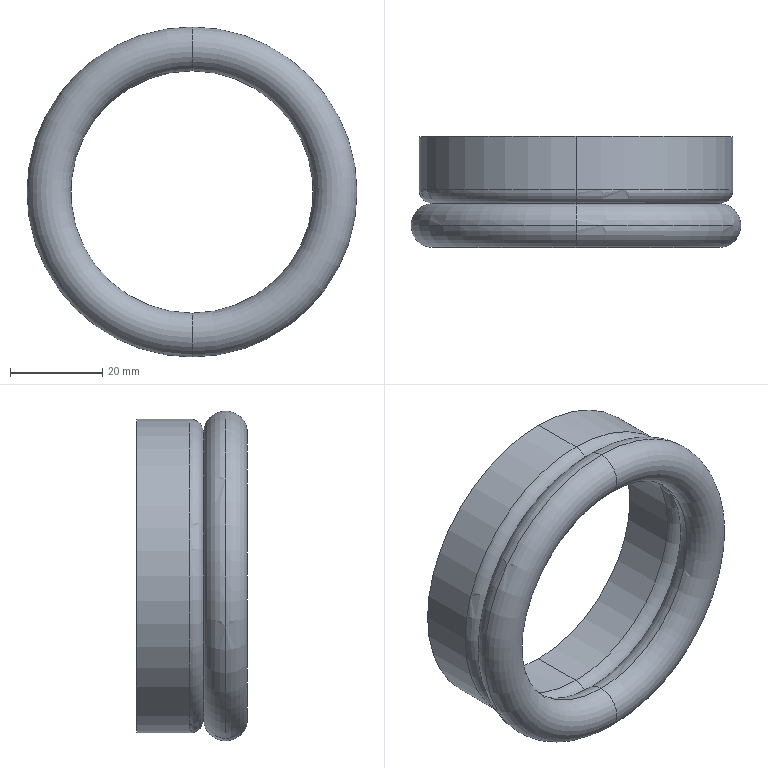Part | SolidWorks | features Sweep 2 | 2 solids | 22 faces | box 71.5 x 24 x 71.5 mm | volume 15845 mm3 | torus 12 | cylinder 8 | plane 2 | commonest cylinder face diameters 56 x2 59.2 x2 64.8 x2 68 x2
STEP:
#1=CARTESIAN_POINT('',(31.,19.25,32.4));
#2=VERTEX_POINT('',#1);
#3=CARTESIAN_POINT('',(31.,19.25,-32.4));
#4=VERTEX_POINT('',#3);
#5=CARTESIAN_POINT('',(31.,19.25,0.));
#6=DIRECTION('',(0.,-1.,0.));
#7=DIRECTION('',(0.,0.,-1.));
#8=AXIS2_PLACEMENT_3D('',#5,#6,#7);
#9=CIRCLE('',#8,32.4);
#10=EDGE_CURVE('',#2,#4,#9,.T.);
#11=ORIENTED_EDGE('',*,*,#10,.F.);
#12=CARTESIAN_POINT('',(31.,7.75,32.4));
#13=VERTEX_POINT('',#12);
#14=CARTESIAN_POINT('',(31.,0.,32.4));
#15=DIRECTION('',(0.,-1.,0.));
#16=VECTOR('',#15,1000.);
#17=LINE('',#14,#16);
#18=EDGE_CURVE('',#2,#13,#17,.T.);
#19=ORIENTED_EDGE('',*,*,#18,.T.);
#20=CARTESIAN_POINT('',(31.,7.75,-32.4));
#21=VERTEX_POINT('',#20);
#22=CARTESIAN_POINT('',(31.,7.75,0.));
#23=DIRECTION('',(0.,-1.,0.));
#24=DIRECTION('',(0.,0.,-1.));
#25=AXIS2_PLACEMENT_3D('',#22,#23,#24);
#26=CIRCLE('',#25,32.4);
#27=EDGE_CURVE('',#13,#21,#26,.T.);
#28=ORIENTED_EDGE('',*,*,#27,.T.);
#29=CARTESIAN_POINT('',(31.,0.,-32.4));
#30=DIRECTION('',(0.,-1.,0.));
#31=VECTOR('',#30,1000.);
#32=LINE('',#29,#31);
#33=EDGE_CURVE('',#4,#21,#32,.T.);
#34=ORIENTED_EDGE('',*,*,#33,.F.);
#35=EDGE_LOOP('',(#11,#19,#28,#34));
#36=FACE_OUTER_BOUND('',#35,.T.);
#37=CARTESIAN_POINT('',(31.,0.,0.));
#38=DIRECTION('',(0.,-1.,0.));
#39=DIRECTION('',(0.,0.,-1.));
#40=AXIS2_PLACEMENT_3D('',#37,#38,#39);
#41=CYLINDRICAL_SURFACE('',#40,32.4);
#42=ADVANCED_FACE('',(#36),#41,.F.);
#43=ORIENTED_EDGE('',*,*,#27,.F.);
#44=CARTESIAN_POINT('',(31.,7.75,29.6));
#45=VERTEX_POINT('',#44);
#46=CARTESIAN_POINT('',(31.,7.75,31.));
#47=DIRECTION('',(1.,0.,0.));
#48=DIRECTION('',(0.,0.,-1.));
#49=AXIS2_PLACEMENT_3D('',#46,#47,#48);
#50=CIRCLE('',#49,1.4);
#51=EDGE_CURVE('',#13,#45,#50,.T.);
#52=ORIENTED_EDGE('',*,*,#51,.T.);
#53=CARTESIAN_POINT('',(31.,7.75,-29.6));
#54=VERTEX_POINT('',#53);
#55=CARTESIAN_POINT('',(31.,7.75,0.));
#56=DIRECTION('',(0.,-1.,0.));
#57=DIRECTION('',(0.,0.,-1.));
#58=AXIS2_PLACEMENT_3D('',#55,#56,#57);
#59=CIRCLE('',#58,29.6);
#60=EDGE_CURVE('',#45,#54,#59,.T.);
#61=ORIENTED_EDGE('',*,*,#60,.T.);
#62=CARTESIAN_POINT('',(31.,7.75,-31.));
#63=DIRECTION('',(-1.,0.,0.));
#64=DIRECTION('',(0.,0.,1.));
#65=AXIS2_PLACEMENT_3D('',#62,#63,#64);
#66=CIRCLE('',#65,1.4);
#67=EDGE_CURVE('',#21,#54,#66,.T.);
#68=ORIENTED_EDGE('',*,*,#67,.F.);
#69=EDGE_LOOP('',(#43,#52,#61,#68));
#70=FACE_OUTER_BOUND('',#69,.T.);
#71=CARTESIAN_POINT('',(31.,7.75,0.));
#72=DIRECTION('',(0.,-1.,0.));
#73=DIRECTION('',(0.,0.,-1.));
#74=AXIS2_PLACEMENT_3D('',#71,#72,#73);
#75=TOROIDAL_SURFACE('',#74,31.,1.4);
#76=ADVANCED_FACE('',(#70),#75,.F.);
#77=CARTESIAN_POINT('',(31.,19.25,-29.6));
#78=VERTEX_POINT('',#77);
#79=CARTESIAN_POINT('',(31.,19.25,29.6));
#80=VERTEX_POINT('',#79);
#81=CARTESIAN_POINT('',(31.,19.25,0.));
#82=DIRECTION('',(0.,-1.,0.));
#83=DIRECTION('',(0.,0.,-1.));
#84=AXIS2_PLACEMENT_3D('',#81,#82,#83);
#85=CIRCLE('',#84,29.6);
#86=EDGE_CURVE('',#78,#80,#85,.T.);
#87=ORIENTED_EDGE('',*,*,#86,.T.);
#88=CARTESIAN_POINT('',(31.,0.,29.6));
#89=DIRECTION('',(0.,-1.,0.));
#90=VECTOR('',#89,1000.);
#91=LINE('',#88,#90);
#92=EDGE_CURVE('',#80,#45,#91,.T.);
#93=ORIENTED_EDGE('',*,*,#92,.T.);
#94=CARTESIAN_POINT('',(31.,7.75,0.));
#95=DIRECTION('',(0.,-1.,0.));
#96=DIRECTION('',(0.,0.,-1.));
#97=AXIS2_PLACEMENT_3D('',#94,#95,#96);
#98=CIRCLE('',#97,29.6);
#99=EDGE_CURVE('',#54,#45,#98,.T.);
#100=ORIENTED_EDGE('',*,*,#99,.F.);
#101=CARTESIAN_POINT('',(31.,0.,-29.6));
#102=DIRECTION('',(0.,-1.,0.));
#103=VECTOR('',#102,1000.);
#104=LINE('',#101,#103);
#105=EDGE_CURVE('',#78,#54,#104,.T.);
#106=ORIENTED_EDGE('',*,*,#105,.F.);
#107=EDGE_LOOP('',(#87,#93,#100,#106));
#108=FACE_OUTER_BOUND('',#107,.T.);
#109=CARTESIAN_POINT('',(31.,0.,0.));
#110=DIRECTION('',(0.,-1.,0.));
#111=DIRECTION('',(0.,0.,-1.));
#112=AXIS2_PLACEMENT_3D('',#109,#110,#111);
#113=CYLINDRICAL_SURFACE('',#112,29.6);
#114=ADVANCED_FACE('',(#108),#113,.T.);
#115=CARTESIAN_POINT('',(31.,19.25,28.));
#116=VERTEX_POINT('',#115);
#117=CARTESIAN_POINT('',(31.,19.25,-28.));
#118=VERTEX_POINT('',#117);
#119=CARTESIAN_POINT('',(31.,19.25,0.));
#120=DIRECTION('',(0.,-1.,0.));
#121=DIRECTION('',(0.,0.,-1.));
#122=AXIS2_PLACEMENT_3D('',#119,#120,#121);
#123=CIRCLE('',#122,28.);
#124=EDGE_CURVE('',#116,#118,#123,.T.);
#125=ORIENTED_EDGE('',*,*,#124,.F.);
#126=CARTESIAN_POINT('',(31.,7.75,28.));
#127=VERTEX_POINT('',#126);
#128=CARTESIAN_POINT('',(31.,0.,28.));
#129=DIRECTION('',(0.,-1.,0.));
#130=VECTOR('',#129,1000.);
#131=LINE('',#128,#130);
#132=EDGE_CURVE('',#116,#127,#131,.T.);
#133=ORIENTED_EDGE('',*,*,#132,.T.);
#134=CARTESIAN_POINT('',(31.,7.75,-28.));
#135=VERTEX_POINT('',#134);
#136=CARTESIAN_POINT('',(31.,7.75,0.));
#137=DIRECTION('',(0.,-1.,0.));
#138=DIRECTION('',(0.,0.,-1.));
#139=AXIS2_PLACEMENT_3D('',#136,#137,#138);
#140=CIRCLE('',#139,28.);
#141=EDGE_CURVE('',#127,#135,#140,.T.);
#142=ORIENTED_EDGE('',*,*,#141,.T.);
#143=CARTESIAN_POINT('',(31.,0.,-28.));
#144=DIRECTION('',(0.,-1.,0.));
#145=VECTOR('',#144,1000.);
#146=LINE('',#143,#145);
#147=EDGE_CURVE('',#118,#135,#146,.T.);
#148=ORIENTED_EDGE('',*,*,#147,.F.);
#149=EDGE_LOOP('',(#125,#133,#142,#148));
#150=FACE_OUTER_BOUND('',#149,.T.);
#151=CARTESIAN_POINT('',(31.,0.,0.));
#152=DIRECTION('',(0.,-1.,0.));
#153=DIRECTION('',(0.,0.,-1.));
#154=AXIS2_PLACEMENT_3D('',#151,#152,#153);
#155=CYLINDRICAL_SURFACE('',#154,28.);
#156=ADVANCED_FACE('',(#150),#155,.F.);
#157=CARTESIAN_POINT('',(31.,7.75,-34.));
#158=VERTEX_POINT('',#157);
#159=CARTESIAN_POINT('',(31.,7.75,34.));
#160=VERTEX_POINT('',#159);
#161=CARTESIAN_POINT('',(31.,7.75,0.));
#162=DIRECTION('',(0.,-1.,0.));
#163=DIRECTION('',(0.,0.,-1.));
#164=AXIS2_PLACEMENT_3D('',#161,#162,#163);
#165=CIRCLE('',#164,34.);
#166=EDGE_CURVE('',#158,#160,#165,.T.);
#167=ORIENTED_EDGE('',*,*,#166,.T.);
#168=CARTESIAN_POINT('',(31.,7.75,31.));
#169=DIRECTION('',(1.,0.,0.));
#170=DIRECTION('',(0.,0.,-1.));
#171=AXIS2_PLACEMENT_3D('',#168,#169,#170);
#172=CIRCLE('',#171,3.);
#173=EDGE_CURVE('',#160,#127,#172,.T.);
#174=ORIENTED_EDGE('',*,*,#173,.T.);
#175=CARTESIAN_POINT('',(31.,7.75,0.));
#176=DIRECTION('',(0.,-1.,0.));
#177=DIRECTION('',(0.,0.,-1.));
#178=AXIS2_PLACEMENT_3D('',#175,#176,#177);
#179=CIRCLE('',#178,28.);
#180=EDGE_CURVE('',#135,#127,#179,.T.);
#181=ORIENTED_EDGE('',*,*,#180,.F.);
#182=CARTESIAN_POINT('',(31.,7.75,-31.));
#183=DIRECTION('',(-1.,0.,0.));
#184=DIRECTION('',(0.,0.,1.));
#185=AXIS2_PLACEMENT_3D('',#182,#183,#184);
#186=CIRCLE('',#185,3.);
#187=EDGE_CURVE('',#158,#135,#186,.T.);
#188=ORIENTED_EDGE('',*,*,#187,.F.);
#189=EDGE_LOOP('',(#167,#174,#181,#188));
#190=FACE_OUTER_BOUND('',#189,.T.);
#191=CARTESIAN_POINT('',(31.,7.75,0.));
#192=DIRECTION('',(0.,-1.,0.));
#193=DIRECTION('',(0.,0.,-1.));
#194=AXIS2_PLACEMENT_3D('',#191,#192,#193);
#195=TOROIDAL_SURFACE('',#194,31.,3.);
#196=ADVANCED_FACE('',(#190),#195,.T.);
#197=CARTESIAN_POINT('',(31.,19.25,-34.));
#198=VERTEX_POINT('',#197);
#199=CARTESIAN_POINT('',(31.,19.25,34.));
#200=VERTEX_POINT('',#199);
#201=CARTESIAN_POINT('',(31.,19.25,0.));
#202=DIRECTION('',(0.,-1.,0.));
#203=DIRECTION('',(0.,0.,-1.));
#204=AXIS2_PLACEMENT_3D('',#201,#202,#203);
#205=CIRCLE('',#204,34.);
#206=EDGE_CURVE('',#198,#200,#205,.T.);
#207=ORIENTED_EDGE('',*,*,#206,.T.);
#208=CARTESIAN_POINT('',(31.,0.,34.));
#209=DIRECTION('',(0.,-1.,0.));
#210=VECTOR('',#209,1000.);
#211=LINE('',#208,#210);
#212=EDGE_CURVE('',#200,#160,#211,.T.);
#213=ORIENTED_EDGE('',*,*,#212,.T.);
#214=ORIENTED_EDGE('',*,*,#166,.F.);
#215=CARTESIAN_POINT('',(31.,0.,-34.));
#216=DIRECTION('',(0.,-1.,0.));
#217=VECTOR('',#216,1000.);
#218=LINE('',#215,#217);
#219=EDGE_CURVE('',#198,#158,#218,.T.);
#220=ORIENTED_EDGE('',*,*,#219,.F.);
#221=EDGE_LOOP('',(#207,#213,#214,#220));
#222=FACE_OUTER_BOUND('',#221,.T.);
#223=CARTESIAN_POINT('',(31.,0.,0.));
#224=DIRECTION('',(0.,-1.,0.));
#225=DIRECTION('',(0.,0.,-1.));
#226=AXIS2_PLACEMENT_3D('',#223,#224,#225);
#227=CYLINDRICAL_SURFACE('',#226,34.);
#228=ADVANCED_FACE('',(#222),#227,.T.);
#229=ORIENTED_EDGE('',*,*,#206,.F.);
#230=CARTESIAN_POINT('',(31.,19.25,0.));
#231=DIRECTION('',(0.,-1.,0.));
#232=DIRECTION('',(0.,0.,-1.));
#233=AXIS2_PLACEMENT_3D('',#230,#231,#232);
#234=CIRCLE('',#233,34.);
#235=EDGE_CURVE('',#200,#198,#234,.T.);
#236=ORIENTED_EDGE('',*,*,#235,.F.);
#237=EDGE_LOOP('',(#229,#236));
#238=FACE_OUTER_BOUND('',#237,.T.);
#239=CARTESIAN_POINT('',(31.,19.25,0.));
#240=DIRECTION('',(0.,-1.,0.));
#241=DIRECTION('',(0.,0.,-1.));
#242=AXIS2_PLACEMENT_3D('',#239,#240,#241);
#243=CIRCLE('',#242,32.4);
#244=EDGE_CURVE('',#4,#2,#243,.T.);
#245=ORIENTED_EDGE('',*,*,#244,.T.);
#246=ORIENTED_EDGE('',*,*,#10,.T.);
#247=EDGE_LOOP('',(#245,#246));
#248=FACE_BOUND('',#247,.T.);
#249=CARTESIAN_POINT('',(-3.,19.25,0.));
#250=DIRECTION('',(0.,-1.,0.));
#251=DIRECTION('',(0.,0.,-1.));
#252=AXIS2_PLACEMENT_3D('',#249,#250,#251);
#253=PLANE('',#252);
#254=ADVANCED_FACE('',(#238,#248),#253,.F.);
#255=ORIENTED_EDGE('',*,*,#212,.F.);
#256=ORIENTED_EDGE('',*,*,#235,.T.);
#257=ORIENTED_EDGE('',*,*,#219,.T.);
#258=CARTESIAN_POINT('',(31.,7.75,0.));
#259=DIRECTION('',(0.,-1.,0.));
#260=DIRECTION('',(0.,0.,-1.));
#261=AXIS2_PLACEMENT_3D('',#258,#259,#260);
#262=CIRCLE('',#261,34.);
#263=EDGE_CURVE('',#160,#158,#262,.T.);
#264=ORIENTED_EDGE('',*,*,#263,.F.);
#265=EDGE_LOOP('',(#255,#256,#257,#264));
#266=FACE_OUTER_BOUND('',#265,.T.);
#267=CARTESIAN_POINT('',(31.,0.,0.));
#268=DIRECTION('',(0.,-1.,0.));
#269=DIRECTION('',(0.,0.,-1.));
#270=AXIS2_PLACEMENT_3D('',#267,#268,#269);
#271=CYLINDRICAL_SURFACE('',#270,34.);
#272=ADVANCED_FACE('',(#266),#271,.T.);
#273=ORIENTED_EDGE('',*,*,#173,.F.);
#274=ORIENTED_EDGE('',*,*,#263,.T.);
#275=ORIENTED_EDGE('',*,*,#187,.T.);
#276=ORIENTED_EDGE('',*,*,#141,.F.);
#277=EDGE_LOOP('',(#273,#274,#275,#276));
#278=FACE_OUTER_BOUND('',#277,.T.);
#279=CARTESIAN_POINT('',(31.,7.75,0.));
#280=DIRECTION('',(0.,-1.,0.));
#281=DIRECTION('',(0.,0.,-1.));
#282=AXIS2_PLACEMENT_3D('',#279,#280,#281);
#283=TOROIDAL_SURFACE('',#282,31.,3.);
#284=ADVANCED_FACE('',(#278),#283,.T.);
#285=ORIENTED_EDGE('',*,*,#132,.F.);
#286=CARTESIAN_POINT('',(31.,19.25,0.));
#287=DIRECTION('',(0.,-1.,0.));
#288=DIRECTION('',(0.,0.,-1.));
#289=AXIS2_PLACEMENT_3D('',#286,#287,#288);
#290=CIRCLE('',#289,28.);
#291=EDGE_CURVE('',#118,#116,#290,.T.);
#292=ORIENTED_EDGE('',*,*,#291,.F.);
#293=ORIENTED_EDGE('',*,*,#147,.T.);
#294=ORIENTED_EDGE('',*,*,#180,.T.);
#295=EDGE_LOOP('',(#285,#292,#293,#294));
#296=FACE_OUTER_BOUND('',#295,.T.);
#297=CARTESIAN_POINT('',(31.,0.,0.));
#298=DIRECTION('',(0.,-1.,0.));
#299=DIRECTION('',(0.,0.,-1.));
#300=AXIS2_PLACEMENT_3D('',#297,#298,#299);
#301=CYLINDRICAL_SURFACE('',#300,28.);
#302=ADVANCED_FACE('',(#296),#301,.F.);
#303=ORIENTED_EDGE('',*,*,#86,.F.);
#304=CARTESIAN_POINT('',(31.,19.25,0.));
#305=DIRECTION('',(0.,-1.,0.));
#306=DIRECTION('',(0.,0.,-1.));
#307=AXIS2_PLACEMENT_3D('',#304,#305,#306);
#308=CIRCLE('',#307,29.6);
#309=EDGE_CURVE('',#80,#78,#308,.T.);
#310=ORIENTED_EDGE('',*,*,#309,.F.);
#311=EDGE_LOOP('',(#303,#310));
#312=FACE_OUTER_BOUND('',#311,.T.);
#313=ORIENTED_EDGE('',*,*,#291,.T.);
#314=ORIENTED_EDGE('',*,*,#124,.T.);
#315=EDGE_LOOP('',(#313,#314));
#316=FACE_BOUND('',#315,.T.);
#317=CARTESIAN_POINT('',(1.4,19.25,0.));
#318=DIRECTION('',(0.,-1.,0.));
#319=DIRECTION('',(0.,0.,-1.));
#320=AXIS2_PLACEMENT_3D('',#317,#318,#319);
#321=PLANE('',#320);
#322=ADVANCED_FACE('',(#312,#316),#321,.F.);
#323=ORIENTED_EDGE('',*,*,#92,.F.);
#324=ORIENTED_EDGE('',*,*,#309,.T.);
#325=ORIENTED_EDGE('',*,*,#105,.T.);
#326=ORIENTED_EDGE('',*,*,#60,.F.);
#327=EDGE_LOOP('',(#323,#324,#325,#326));
#328=FACE_OUTER_BOUND('',#327,.T.);
#329=CARTESIAN_POINT('',(31.,0.,0.));
#330=DIRECTION('',(0.,-1.,0.));
#331=DIRECTION('',(0.,0.,-1.));
#332=AXIS2_PLACEMENT_3D('',#329,#330,#331);
#333=CYLINDRICAL_SURFACE('',#332,29.6);
#334=ADVANCED_FACE('',(#328),#333,.T.);
#335=ORIENTED_EDGE('',*,*,#51,.F.);
#336=CARTESIAN_POINT('',(31.,7.75,0.));
#337=DIRECTION('',(0.,-1.,0.));
#338=DIRECTION('',(0.,0.,-1.));
#339=AXIS2_PLACEMENT_3D('',#336,#337,#338);
#340=CIRCLE('',#339,32.4);
#341=EDGE_CURVE('',#21,#13,#340,.T.);
#342=ORIENTED_EDGE('',*,*,#341,.F.);
#343=ORIENTED_EDGE('',*,*,#67,.T.);
#344=ORIENTED_EDGE('',*,*,#99,.T.);
#345=EDGE_LOOP('',(#335,#342,#343,#344));
#346=FACE_OUTER_BOUND('',#345,.T.);
#347=CARTESIAN_POINT('',(31.,7.75,0.));
#348=DIRECTION('',(0.,-1.,0.));
#349=DIRECTION('',(0.,0.,-1.));
#350=AXIS2_PLACEMENT_3D('',#347,#348,#349);
#351=TOROIDAL_SURFACE('',#350,31.,1.4);
#352=ADVANCED_FACE('',(#346),#351,.F.);
#353=ORIENTED_EDGE('',*,*,#18,.F.);
#354=ORIENTED_EDGE('',*,*,#244,.F.);
#355=ORIENTED_EDGE('',*,*,#33,.T.);
#356=ORIENTED_EDGE('',*,*,#341,.T.);
#357=EDGE_LOOP('',(#353,#354,#355,#356));
#358=FACE_OUTER_BOUND('',#357,.T.);
#359=CARTESIAN_POINT('',(31.,0.,0.));
#360=DIRECTION('',(0.,-1.,0.));
#361=DIRECTION('',(0.,0.,-1.));
#362=AXIS2_PLACEMENT_3D('',#359,#360,#361);
#363=CYLINDRICAL_SURFACE('',#362,32.4);
#364=ADVANCED_FACE('',(#358),#363,.F.);
#365=CLOSED_SHELL('',(#42,#76,#114,#156,#196,#228,#254,#272,#284,#302,#322,#334,#352,#364));
#366=MANIFOLD_SOLID_BREP('',#365);
#367=CARTESIAN_POINT('',(31.,0.,35.75));
#368=VERTEX_POINT('',#367);
#369=CARTESIAN_POINT('',(31.,0.,26.25));
#370=VERTEX_POINT('',#369);
#371=CARTESIAN_POINT('',(31.,0.,31.));
#372=DIRECTION('',(1.,0.,0.));
#373=DIRECTION('',(0.,0.,-1.));
#374=AXIS2_PLACEMENT_3D('',#371,#372,#373);
#375=CIRCLE('',#374,4.75);
#376=EDGE_CURVE('',#368,#370,#375,.T.);
#377=ORIENTED_EDGE('',*,*,#376,.F.);
#378=CARTESIAN_POINT('',(31.,0.,-35.75));
#379=VERTEX_POINT('',#378);
#380=CARTESIAN_POINT('',(31.,0.,0.));
#381=DIRECTION('',(0.,-1.,0.));
#382=DIRECTION('',(0.,0.,-1.));
#383=AXIS2_PLACEMENT_3D('',#380,#381,#382);
#384=CIRCLE('',#383,35.75);
#385=EDGE_CURVE('',#368,#379,#384,.T.);
#386=ORIENTED_EDGE('',*,*,#385,.T.);
#387=CARTESIAN_POINT('',(31.,0.,-26.25));
#388=VERTEX_POINT('',#387);
#389=CARTESIAN_POINT('',(31.,0.,-31.));
#390=DIRECTION('',(-1.,0.,0.));
#391=DIRECTION('',(0.,0.,1.));
#392=AXIS2_PLACEMENT_3D('',#389,#390,#391);
#393=CIRCLE('',#392,4.75);
#394=EDGE_CURVE('',#379,#388,#393,.T.);
#395=ORIENTED_EDGE('',*,*,#394,.T.);
#396=CARTESIAN_POINT('',(31.,0.,0.));
#397=DIRECTION('',(0.,-1.,0.));
#398=DIRECTION('',(0.,0.,-1.));
#399=AXIS2_PLACEMENT_3D('',#396,#397,#398);
#400=CIRCLE('',#399,26.25);
#401=EDGE_CURVE('',#370,#388,#400,.T.);
#402=ORIENTED_EDGE('',*,*,#401,.F.);
#403=EDGE_LOOP('',(#377,#386,#395,#402));
#404=FACE_OUTER_BOUND('',#403,.T.);
#405=CARTESIAN_POINT('',(31.,0.,0.));
#406=DIRECTION('',(0.,-1.,0.));
#407=DIRECTION('',(0.,0.,-1.));
#408=AXIS2_PLACEMENT_3D('',#405,#406,#407);
#409=TOROIDAL_SURFACE('',#408,31.,4.75);
#410=ADVANCED_FACE('',(#404),#409,.T.);
#411=ORIENTED_EDGE('',*,*,#394,.F.);
#412=CARTESIAN_POINT('',(31.,0.,0.));
#413=DIRECTION('',(0.,-1.,0.));
#414=DIRECTION('',(0.,0.,-1.));
#415=AXIS2_PLACEMENT_3D('',#412,#413,#414);
#416=CIRCLE('',#415,35.75);
#417=EDGE_CURVE('',#379,#368,#416,.T.);
#418=ORIENTED_EDGE('',*,*,#417,.T.);
#419=ORIENTED_EDGE('',*,*,#376,.T.);
#420=CARTESIAN_POINT('',(31.,0.,0.));
#421=DIRECTION('',(0.,-1.,0.));
#422=DIRECTION('',(0.,0.,-1.));
#423=AXIS2_PLACEMENT_3D('',#420,#421,#422);
#424=CIRCLE('',#423,26.25);
#425=EDGE_CURVE('',#388,#370,#424,.T.);
#426=ORIENTED_EDGE('',*,*,#425,.F.);
#427=EDGE_LOOP('',(#411,#418,#419,#426));
#428=FACE_OUTER_BOUND('',#427,.T.);
#429=CARTESIAN_POINT('',(31.,0.,0.));
#430=DIRECTION('',(0.,-1.,0.));
#431=DIRECTION('',(0.,0.,-1.));
#432=AXIS2_PLACEMENT_3D('',#429,#430,#431);
#433=TOROIDAL_SURFACE('',#432,31.,4.75);
#434=ADVANCED_FACE('',(#428),#433,.T.);
#435=ORIENTED_EDGE('',*,*,#417,.F.);
#436=CARTESIAN_POINT('',(31.,0.,-31.));
#437=DIRECTION('',(-1.,0.,0.));
#438=DIRECTION('',(0.,0.,1.));
#439=AXIS2_PLACEMENT_3D('',#436,#437,#438);
#440=CIRCLE('',#439,4.75);
#441=EDGE_CURVE('',#388,#379,#440,.T.);
#442=ORIENTED_EDGE('',*,*,#441,.F.);
#443=ORIENTED_EDGE('',*,*,#425,.T.);
#444=CARTESIAN_POINT('',(31.,0.,31.));
#445=DIRECTION('',(1.,0.,0.));
#446=DIRECTION('',(0.,0.,-1.));
#447=AXIS2_PLACEMENT_3D('',#444,#445,#446);
#448=CIRCLE('',#447,4.75);
#449=EDGE_CURVE('',#370,#368,#448,.T.);
#450=ORIENTED_EDGE('',*,*,#449,.T.);
#451=EDGE_LOOP('',(#435,#442,#443,#450));
#452=FACE_OUTER_BOUND('',#451,.T.);
#453=CARTESIAN_POINT('',(31.,0.,0.));
#454=DIRECTION('',(0.,-1.,0.));
#455=DIRECTION('',(0.,0.,-1.));
#456=AXIS2_PLACEMENT_3D('',#453,#454,#455);
#457=TOROIDAL_SURFACE('',#456,31.,4.75);
#458=ADVANCED_FACE('',(#452),#457,.T.);
#459=ORIENTED_EDGE('',*,*,#385,.F.);
#460=ORIENTED_EDGE('',*,*,#449,.F.);
#461=ORIENTED_EDGE('',*,*,#401,.T.);
#462=ORIENTED_EDGE('',*,*,#441,.T.);
#463=EDGE_LOOP('',(#459,#460,#461,#462));
#464=FACE_OUTER_BOUND('',#463,.T.);
#465=CARTESIAN_POINT('',(31.,0.,0.));
#466=DIRECTION('',(0.,-1.,0.));
#467=DIRECTION('',(0.,0.,-1.));
#468=AXIS2_PLACEMENT_3D('',#465,#466,#467);
#469=TOROIDAL_SURFACE('',#468,31.,4.75);
#470=ADVANCED_FACE('',(#464),#469,.T.);
#471=CLOSED_SHELL('',(#410,#434,#458,#470));
#472=CARTESIAN_POINT('',(31.,0.,-27.55));
#473=VERTEX_POINT('',#472);
#474=CARTESIAN_POINT('',(31.,0.,-34.45));
#475=VERTEX_POINT('',#474);
#476=CARTESIAN_POINT('',(31.,0.,-31.));
#477=DIRECTION('',(-1.,0.,0.));
#478=DIRECTION('',(0.,0.,1.));
#479=AXIS2_PLACEMENT_3D('',#476,#477,#478);
#480=CIRCLE('',#479,3.45);
#481=EDGE_CURVE('',#473,#475,#480,.T.);
#482=ORIENTED_EDGE('',*,*,#481,.T.);
#483=CARTESIAN_POINT('',(31.,0.,34.45));
#484=VERTEX_POINT('',#483);
#485=CARTESIAN_POINT('',(31.,0.,0.));
#486=DIRECTION('',(0.,-1.,0.));
#487=DIRECTION('',(0.,0.,-1.));
#488=AXIS2_PLACEMENT_3D('',#485,#486,#487);
#489=CIRCLE('',#488,34.45);
#490=EDGE_CURVE('',#475,#484,#489,.T.);
#491=ORIENTED_EDGE('',*,*,#490,.T.);
#492=CARTESIAN_POINT('',(31.,0.,27.55));
#493=VERTEX_POINT('',#492);
#494=CARTESIAN_POINT('',(31.,0.,31.));
#495=DIRECTION('',(1.,0.,0.));
#496=DIRECTION('',(0.,0.,-1.));
#497=AXIS2_PLACEMENT_3D('',#494,#495,#496);
#498=CIRCLE('',#497,3.45);
#499=EDGE_CURVE('',#493,#484,#498,.T.);
#500=ORIENTED_EDGE('',*,*,#499,.F.);
#501=CARTESIAN_POINT('',(31.,0.,0.));
#502=DIRECTION('',(0.,-1.,0.));
#503=DIRECTION('',(0.,0.,-1.));
#504=AXIS2_PLACEMENT_3D('',#501,#502,#503);
#505=CIRCLE('',#504,27.55);
#506=EDGE_CURVE('',#473,#493,#505,.T.);
#507=ORIENTED_EDGE('',*,*,#506,.F.);
#508=EDGE_LOOP('',(#482,#491,#500,#507));
#509=FACE_OUTER_BOUND('',#508,.T.);
#510=CARTESIAN_POINT('',(31.,0.,0.));
#511=DIRECTION('',(0.,-1.,0.));
#512=DIRECTION('',(0.,0.,-1.));
#513=AXIS2_PLACEMENT_3D('',#510,#511,#512);
#514=TOROIDAL_SURFACE('',#513,31.,3.45);
#515=ADVANCED_FACE('',(#509),#514,.F.);
#516=ORIENTED_EDGE('',*,*,#499,.T.);
#517=CARTESIAN_POINT('',(31.,0.,0.));
#518=DIRECTION('',(0.,-1.,0.));
#519=DIRECTION('',(0.,0.,-1.));
#520=AXIS2_PLACEMENT_3D('',#517,#518,#519);
#521=CIRCLE('',#520,34.45);
#522=EDGE_CURVE('',#484,#475,#521,.T.);
#523=ORIENTED_EDGE('',*,*,#522,.T.);
#524=ORIENTED_EDGE('',*,*,#481,.F.);
#525=CARTESIAN_POINT('',(31.,0.,0.));
#526=DIRECTION('',(0.,-1.,0.));
#527=DIRECTION('',(0.,0.,-1.));
#528=AXIS2_PLACEMENT_3D('',#525,#526,#527);
#529=CIRCLE('',#528,27.55);
#530=EDGE_CURVE('',#493,#473,#529,.T.);
#531=ORIENTED_EDGE('',*,*,#530,.F.);
#532=EDGE_LOOP('',(#516,#523,#524,#531));
#533=FACE_OUTER_BOUND('',#532,.T.);
#534=CARTESIAN_POINT('',(31.,0.,0.));
#535=DIRECTION('',(0.,-1.,0.));
#536=DIRECTION('',(0.,0.,-1.));
#537=AXIS2_PLACEMENT_3D('',#534,#535,#536);
#538=TOROIDAL_SURFACE('',#537,31.,3.45);
#539=ADVANCED_FACE('',(#533),#538,.F.);
#540=ORIENTED_EDGE('',*,*,#522,.F.);
#541=CARTESIAN_POINT('',(31.,0.,31.));
#542=DIRECTION('',(1.,0.,0.));
#543=DIRECTION('',(0.,0.,-1.));
#544=AXIS2_PLACEMENT_3D('',#541,#542,#543);
#545=CIRCLE('',#544,3.45);
#546=EDGE_CURVE('',#484,#493,#545,.T.);
#547=ORIENTED_EDGE('',*,*,#546,.T.);
#548=ORIENTED_EDGE('',*,*,#530,.T.);
#549=CARTESIAN_POINT('',(31.,0.,-31.));
#550=DIRECTION('',(-1.,0.,0.));
#551=DIRECTION('',(0.,0.,1.));
#552=AXIS2_PLACEMENT_3D('',#549,#550,#551);
#553=CIRCLE('',#552,3.45);
#554=EDGE_CURVE('',#475,#473,#553,.T.);
#555=ORIENTED_EDGE('',*,*,#554,.F.);
#556=EDGE_LOOP('',(#540,#547,#548,#555));
#557=FACE_OUTER_BOUND('',#556,.T.);
#558=CARTESIAN_POINT('',(31.,0.,0.));
#559=DIRECTION('',(0.,-1.,0.));
#560=DIRECTION('',(0.,0.,-1.));
#561=AXIS2_PLACEMENT_3D('',#558,#559,#560);
#562=TOROIDAL_SURFACE('',#561,31.,3.45);
#563=ADVANCED_FACE('',(#557),#562,.F.);
#564=ORIENTED_EDGE('',*,*,#490,.F.);
#565=ORIENTED_EDGE('',*,*,#554,.T.);
#566=ORIENTED_EDGE('',*,*,#506,.T.);
#567=ORIENTED_EDGE('',*,*,#546,.F.);
#568=EDGE_LOOP('',(#564,#565,#566,#567));
#569=FACE_OUTER_BOUND('',#568,.T.);
#570=CARTESIAN_POINT('',(31.,0.,0.));
#571=DIRECTION('',(0.,-1.,0.));
#572=DIRECTION('',(0.,0.,-1.));
#573=AXIS2_PLACEMENT_3D('',#570,#571,#572);
#574=TOROIDAL_SURFACE('',#573,31.,3.45);
#575=ADVANCED_FACE('',(#569),#574,.F.);
#576=CLOSED_SHELL('',(#515,#539,#563,#575));
#577=ORIENTED_CLOSED_SHELL('',*,#576,.F.);
#578=BREP_WITH_VOIDS('',#471,(#577));
#579=CARTESIAN_POINT('',(0.,0.,0.));
#580=DIRECTION('',(0.,0.,1.));
#581=DIRECTION('',(1.,0.,0.));
#582=AXIS2_PLACEMENT_3D('',#579,#580,#581);
#583=(LENGTH_UNIT()NAMED_UNIT(*)SI_UNIT(.MILLI.,.METRE.));
#584=UNCERTAINTY_MEASURE_WITH_UNIT(LENGTH_MEASURE(0.00001),#583,'','');
#585=(NAMED_UNIT(*)PLANE_ANGLE_UNIT()SI_UNIT($,.RADIAN.));
#586=(NAMED_UNIT(*)SI_UNIT($,.STERADIAN.)SOLID_ANGLE_UNIT());
#587=(GEOMETRIC_REPRESENTATION_CONTEXT(3)GLOBAL_UNCERTAINTY_ASSIGNED_CONTEXT((#584))GLOBAL_UNIT_ASSIGNED_CONTEXT((#583,#585,#586))REPRESENTATION_CONTEXT('',''));
#588=ADVANCED_BREP_SHAPE_REPRESENTATION('',(#366,#578,#582),#587);